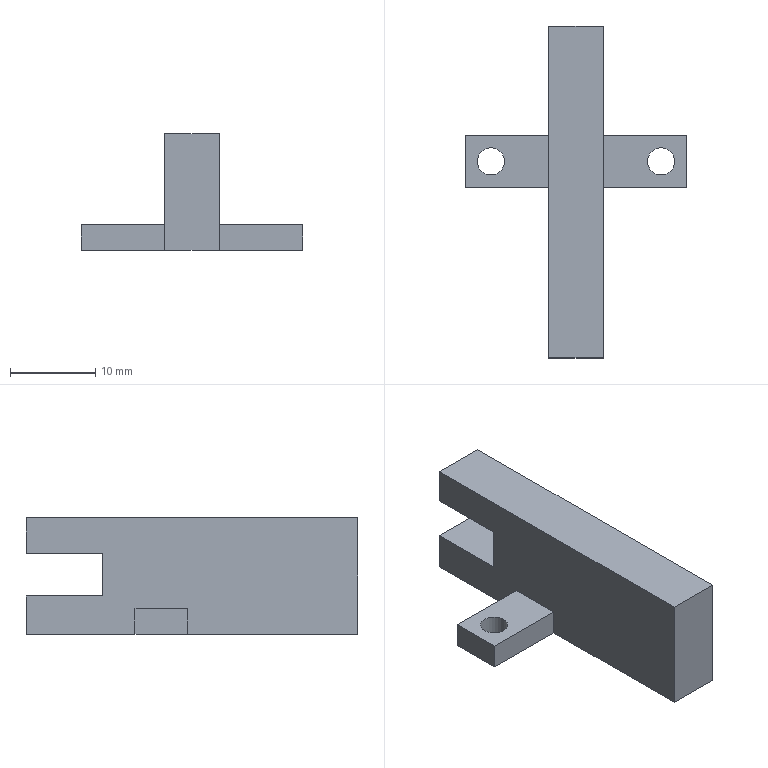Part | NX | 1 solid | 129 faces | box 26 x 39 x 13.7 mm | volume 3422 mm3 | plane 78 | spline 49 | cylinder 2 | commonest cylinder face diameters 3.2 x2